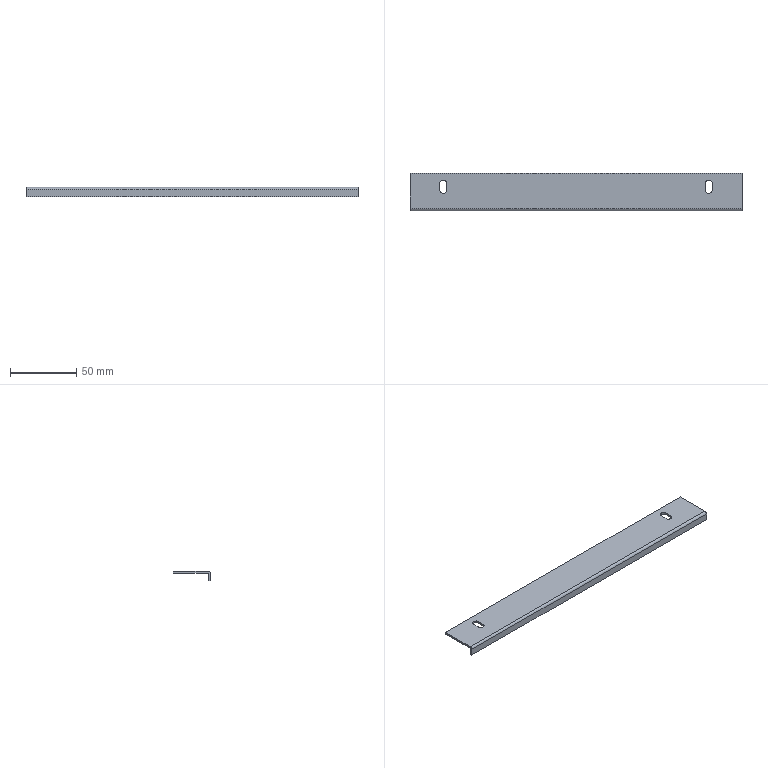Part | STEP file | FHD-021-014-02 acrylic press plate | 1 solid | 18 faces | box 250 x 28 x 7 mm | volume 12276 mm3 | plane 12 | cylinder 6 | commonest cylinder face diameters 5 x4 0.4 x1 3.4 x1
STEP:
#1=CARTESIAN_POINT('',(0.,0.,0.));
#2=DIRECTION('',(0.,0.,1.));
#3=DIRECTION('',(1.,0.,0.));
#4=AXIS2_PLACEMENT_3D('',#1,#2,#3);
#5=CARTESIAN_POINT('',(-125.,-12.3,-1.5));
#6=VERTEX_POINT('',#5);
#7=CARTESIAN_POINT('',(-125.,14.,-1.5));
#8=VERTEX_POINT('',#7);
#9=CARTESIAN_POINT('',(-125.,0.,-1.5));
#10=DIRECTION('',(0.,1.,0.));
#11=VECTOR('',#10,1.);
#12=LINE('',#9,#11);
#13=CARTESIAN_POINT('',(0.,0.,-1.5));
#14=DIRECTION('',(0.,0.,-1.));
#15=DIRECTION('',(-1.,0.,0.));
#16=AXIS2_PLACEMENT_3D('',#13,#14,#15);
#17=PLANE('',#16);
#18=CARTESIAN_POINT('',(125.,0.));
#19=DIRECTION('',(0.,1.));
#20=VECTOR('',#19,1.);
#21=LINE('',#18,#20);
#22=(GEOMETRIC_REPRESENTATION_CONTEXT(2)PARAMETRIC_REPRESENTATION_CONTEXT()REPRESENTATION_CONTEXT('',''));
#23=DEFINITIONAL_REPRESENTATION('',(#21),#22);
#24=PCURVE('',#17,#23);
#25=CARTESIAN_POINT('',(-125.,-14.,-1.5));
#26=DIRECTION('',(-1.,0.,0.));
#27=DIRECTION('',(0.,0.,1.));
#28=AXIS2_PLACEMENT_3D('',#25,#26,#27);
#29=PLANE('',#28);
#30=CARTESIAN_POINT('',(0.,14.));
#31=DIRECTION('',(0.,1.));
#32=VECTOR('',#31,1.);
#33=LINE('',#30,#32);
#34=(GEOMETRIC_REPRESENTATION_CONTEXT(2)PARAMETRIC_REPRESENTATION_CONTEXT()REPRESENTATION_CONTEXT('',''));
#35=DEFINITIONAL_REPRESENTATION('',(#33),#34);
#36=PCURVE('',#29,#35);
#37=SURFACE_CURVE('',#12,(#24,#36),.PCURVE_S1.);
#38=EDGE_CURVE('',#6,#8,#37,.T.);
#39=ORIENTED_EDGE('',*,*,#38,.T.);
#40=CARTESIAN_POINT('',(125.,14.,-1.5));
#41=VERTEX_POINT('',#40);
#42=CARTESIAN_POINT('',(0.,14.,-1.5));
#43=DIRECTION('',(1.,0.,0.));
#44=VECTOR('',#43,1.);
#45=LINE('',#42,#44);
#46=CARTESIAN_POINT('',(0.,14.));
#47=DIRECTION('',(-1.,0.));
#48=VECTOR('',#47,1.);
#49=LINE('',#46,#48);
#50=(GEOMETRIC_REPRESENTATION_CONTEXT(2)PARAMETRIC_REPRESENTATION_CONTEXT()REPRESENTATION_CONTEXT('',''));
#51=DEFINITIONAL_REPRESENTATION('',(#49),#50);
#52=PCURVE('',#17,#51);
#53=CARTESIAN_POINT('',(-125.,14.,-1.5));
#54=DIRECTION('',(0.,1.,0.));
#55=DIRECTION('',(0.,0.,1.));
#56=AXIS2_PLACEMENT_3D('',#53,#54,#55);
#57=PLANE('',#56);
#58=CARTESIAN_POINT('',(0.,125.));
#59=DIRECTION('',(0.,1.));
#60=VECTOR('',#59,1.);
#61=LINE('',#58,#60);
#62=(GEOMETRIC_REPRESENTATION_CONTEXT(2)PARAMETRIC_REPRESENTATION_CONTEXT()REPRESENTATION_CONTEXT('',''));
#63=DEFINITIONAL_REPRESENTATION('',(#61),#62);
#64=PCURVE('',#57,#63);
#65=SURFACE_CURVE('',#45,(#52,#64),.PCURVE_S1.);
#66=EDGE_CURVE('',#8,#41,#65,.T.);
#67=ORIENTED_EDGE('',*,*,#66,.T.);
#68=CARTESIAN_POINT('',(125.,-12.3,-1.5));
#69=VERTEX_POINT('',#68);
#70=CARTESIAN_POINT('',(125.,0.,-1.5));
#71=DIRECTION('',(0.,-1.,0.));
#72=VECTOR('',#71,1.);
#73=LINE('',#70,#72);
#74=CARTESIAN_POINT('',(-125.,0.));
#75=DIRECTION('',(0.,-1.));
#76=VECTOR('',#75,1.);
#77=LINE('',#74,#76);
#78=(GEOMETRIC_REPRESENTATION_CONTEXT(2)PARAMETRIC_REPRESENTATION_CONTEXT()REPRESENTATION_CONTEXT('',''));
#79=DEFINITIONAL_REPRESENTATION('',(#77),#78);
#80=PCURVE('',#17,#79);
#81=CARTESIAN_POINT('',(125.,-14.,-1.5));
#82=DIRECTION('',(1.,0.,0.));
#83=DIRECTION('',(0.,0.,-1.));
#84=AXIS2_PLACEMENT_3D('',#81,#82,#83);
#85=PLANE('',#84);
#86=CARTESIAN_POINT('',(0.,14.));
#87=DIRECTION('',(0.,-1.));
#88=VECTOR('',#87,1.);
#89=LINE('',#86,#88);
#90=(GEOMETRIC_REPRESENTATION_CONTEXT(2)PARAMETRIC_REPRESENTATION_CONTEXT()REPRESENTATION_CONTEXT('',''));
#91=DEFINITIONAL_REPRESENTATION('',(#89),#90);
#92=PCURVE('',#85,#91);
#93=SURFACE_CURVE('',#73,(#80,#92),.PCURVE_S1.);
#94=EDGE_CURVE('',#41,#69,#93,.T.);
#95=ORIENTED_EDGE('',*,*,#94,.T.);
#96=CARTESIAN_POINT('',(0.,-12.3,-1.5));
#97=DIRECTION('',(-1.,0.,0.));
#98=VECTOR('',#97,1.);
#99=LINE('',#96,#98);
#100=CARTESIAN_POINT('',(0.,-12.3));
#101=DIRECTION('',(1.,0.));
#102=VECTOR('',#101,1.);
#103=LINE('',#100,#102);
#104=(GEOMETRIC_REPRESENTATION_CONTEXT(2)PARAMETRIC_REPRESENTATION_CONTEXT()REPRESENTATION_CONTEXT('',''));
#105=DEFINITIONAL_REPRESENTATION('',(#103),#104);
#106=PCURVE('',#17,#105);
#107=CARTESIAN_POINT('',(-125.,-12.3,-1.7));
#108=DIRECTION('',(-1.,0.,0.));
#109=DIRECTION('',(0.,0.,1.));
#110=AXIS2_PLACEMENT_3D('',#107,#108,#109);
#111=CYLINDRICAL_SURFACE('',#110,0.2);
#112=CARTESIAN_POINT('',(6.283,-125.));
#113=DIRECTION('',(0.,1.));
#114=VECTOR('',#113,1.);
#115=LINE('',#112,#114);
#116=(GEOMETRIC_REPRESENTATION_CONTEXT(2)PARAMETRIC_REPRESENTATION_CONTEXT()REPRESENTATION_CONTEXT('',''));
#117=DEFINITIONAL_REPRESENTATION('',(#115),#116);
#118=PCURVE('',#111,#117);
#119=SURFACE_CURVE('',#99,(#106,#118),.PCURVE_S1.);
#120=EDGE_CURVE('',#69,#6,#119,.T.);
#121=ORIENTED_EDGE('',*,*,#120,.T.);
#122=EDGE_LOOP('',(#39,#67,#95,#121));
#123=FACE_BOUND('',#122,.T.);
#124=CARTESIAN_POINT('',(-102.5,1.5,-1.5));
#125=VERTEX_POINT('',#124);
#126=CARTESIAN_POINT('',(-97.5,1.5,-1.5));
#127=VERTEX_POINT('',#126);
#128=CARTESIAN_POINT('',(-100.,1.5,-1.5));
#129=DIRECTION('',(0.,0.,1.));
#130=DIRECTION('',(1.,0.,0.));
#131=AXIS2_PLACEMENT_3D('',#128,#129,#130);
#132=CIRCLE('',#131,2.5);
#133=CARTESIAN_POINT('',(97.5,1.5));
#134=CARTESIAN_POINT('',(97.5,5.83));
#135=CARTESIAN_POINT('',(101.25,3.665));
#136=CARTESIAN_POINT('',(105.,1.5));
#137=CARTESIAN_POINT('',(101.25,-0.6651));
#138=CARTESIAN_POINT('',(97.5,-2.83));
#139=CARTESIAN_POINT('',(97.5,1.5));
#140=(BOUNDED_CURVE()B_SPLINE_CURVE(2,(#133,#134,#135,#136,#137,#138,#139),.UNSPECIFIED.,.T.,.F.)B_SPLINE_CURVE_WITH_KNOTS((1,2,2,2,2,1),(-2.094,0.,2.094,4.189,6.283,8.378),.UNSPECIFIED.)CURVE()GEOMETRIC_REPRESENTATION_ITEM()RATIONAL_B_SPLINE_CURVE((1.,0.5,1.,0.5,1.,0.5,1.))REPRESENTATION_ITEM(''));
#141=(GEOMETRIC_REPRESENTATION_CONTEXT(2)PARAMETRIC_REPRESENTATION_CONTEXT()REPRESENTATION_CONTEXT('',''));
#142=DEFINITIONAL_REPRESENTATION('',(#140),#141);
#143=PCURVE('',#17,#142);
#144=CARTESIAN_POINT('',(-100.,1.5,-10.));
#145=DIRECTION('',(0.,0.,1.));
#146=DIRECTION('',(1.,0.,0.));
#147=AXIS2_PLACEMENT_3D('',#144,#145,#146);
#148=CYLINDRICAL_SURFACE('',#147,2.5);
#149=CARTESIAN_POINT('',(0.,8.5));
#150=DIRECTION('',(1.,0.));
#151=VECTOR('',#150,1.);
#152=LINE('',#149,#151);
#153=(GEOMETRIC_REPRESENTATION_CONTEXT(2)PARAMETRIC_REPRESENTATION_CONTEXT()REPRESENTATION_CONTEXT('',''));
#154=DEFINITIONAL_REPRESENTATION('',(#152),#153);
#155=PCURVE('',#148,#154);
#156=SURFACE_CURVE('',#132,(#143,#155),.PCURVE_S1.);
#157=EDGE_CURVE('',#125,#127,#156,.T.);
#158=ORIENTED_EDGE('',*,*,#157,.T.);
#159=CARTESIAN_POINT('',(-97.5,6.5,-1.5));
#160=VERTEX_POINT('',#159);
#161=CARTESIAN_POINT('',(-97.5,0.,-1.5));
#162=DIRECTION('',(0.,1.,0.));
#163=VECTOR('',#162,1.);
#164=LINE('',#161,#163);
#165=CARTESIAN_POINT('',(97.5,0.));
#166=DIRECTION('',(0.,1.));
#167=VECTOR('',#166,1.);
#168=LINE('',#165,#167);
#169=(GEOMETRIC_REPRESENTATION_CONTEXT(2)PARAMETRIC_REPRESENTATION_CONTEXT()REPRESENTATION_CONTEXT('',''));
#170=DEFINITIONAL_REPRESENTATION('',(#168),#169);
#171=PCURVE('',#17,#170);
#172=CARTESIAN_POINT('',(-97.5,6.5,-10.));
#173=DIRECTION('',(1.,0.,0.));
#174=DIRECTION('',(0.,0.,-1.));
#175=AXIS2_PLACEMENT_3D('',#172,#173,#174);
#176=PLANE('',#175);
#177=CARTESIAN_POINT('',(-8.5,-6.5));
#178=DIRECTION('',(0.,1.));
#179=VECTOR('',#178,1.);
#180=LINE('',#177,#179);
#181=(GEOMETRIC_REPRESENTATION_CONTEXT(2)PARAMETRIC_REPRESENTATION_CONTEXT()REPRESENTATION_CONTEXT('',''));
#182=DEFINITIONAL_REPRESENTATION('',(#180),#181);
#183=PCURVE('',#176,#182);
#184=SURFACE_CURVE('',#164,(#171,#183),.PCURVE_S1.);
#185=EDGE_CURVE('',#127,#160,#184,.T.);
#186=ORIENTED_EDGE('',*,*,#185,.T.);
#187=CARTESIAN_POINT('',(-102.5,6.5,-1.5));
#188=VERTEX_POINT('',#187);
#189=CARTESIAN_POINT('',(-100.,6.5,-1.5));
#190=DIRECTION('',(0.,0.,1.));
#191=DIRECTION('',(1.,0.,0.));
#192=AXIS2_PLACEMENT_3D('',#189,#190,#191);
#193=CIRCLE('',#192,2.5);
#194=CARTESIAN_POINT('',(97.5,6.5));
#195=CARTESIAN_POINT('',(97.5,10.83));
#196=CARTESIAN_POINT('',(101.25,8.665));
#197=CARTESIAN_POINT('',(105.,6.5));
#198=CARTESIAN_POINT('',(101.25,4.335));
#199=CARTESIAN_POINT('',(97.5,2.17));
#200=CARTESIAN_POINT('',(97.5,6.5));
#201=(BOUNDED_CURVE()B_SPLINE_CURVE(2,(#194,#195,#196,#197,#198,#199,#200),.UNSPECIFIED.,.T.,.F.)B_SPLINE_CURVE_WITH_KNOTS((1,2,2,2,2,1),(-2.094,0.,2.094,4.189,6.283,8.378),.UNSPECIFIED.)CURVE()GEOMETRIC_REPRESENTATION_ITEM()RATIONAL_B_SPLINE_CURVE((1.,0.5,1.,0.5,1.,0.5,1.))REPRESENTATION_ITEM(''));
#202=(GEOMETRIC_REPRESENTATION_CONTEXT(2)PARAMETRIC_REPRESENTATION_CONTEXT()REPRESENTATION_CONTEXT('',''));
#203=DEFINITIONAL_REPRESENTATION('',(#201),#202);
#204=PCURVE('',#17,#203);
#205=CARTESIAN_POINT('',(-100.,6.5,-10.));
#206=DIRECTION('',(0.,0.,1.));
#207=DIRECTION('',(1.,0.,0.));
#208=AXIS2_PLACEMENT_3D('',#205,#206,#207);
#209=CYLINDRICAL_SURFACE('',#208,2.5);
#210=CARTESIAN_POINT('',(0.,8.5));
#211=DIRECTION('',(1.,0.));
#212=VECTOR('',#211,1.);
#213=LINE('',#210,#212);
#214=(GEOMETRIC_REPRESENTATION_CONTEXT(2)PARAMETRIC_REPRESENTATION_CONTEXT()REPRESENTATION_CONTEXT('',''));
#215=DEFINITIONAL_REPRESENTATION('',(#213),#214);
#216=PCURVE('',#209,#215);
#217=SURFACE_CURVE('',#193,(#204,#216),.PCURVE_S1.);
#218=EDGE_CURVE('',#160,#188,#217,.T.);
#219=ORIENTED_EDGE('',*,*,#218,.T.);
#220=CARTESIAN_POINT('',(-102.5,0.,-1.5));
#221=DIRECTION('',(0.,-1.,0.));
#222=VECTOR('',#221,1.);
#223=LINE('',#220,#222);
#224=CARTESIAN_POINT('',(102.5,0.));
#225=DIRECTION('',(0.,-1.));
#226=VECTOR('',#225,1.);
#227=LINE('',#224,#226);
#228=(GEOMETRIC_REPRESENTATION_CONTEXT(2)PARAMETRIC_REPRESENTATION_CONTEXT()REPRESENTATION_CONTEXT('',''));
#229=DEFINITIONAL_REPRESENTATION('',(#227),#228);
#230=PCURVE('',#17,#229);
#231=CARTESIAN_POINT('',(-102.5,6.5,-10.));
#232=DIRECTION('',(-1.,0.,0.));
#233=DIRECTION('',(0.,0.,1.));
#234=AXIS2_PLACEMENT_3D('',#231,#232,#233);
#235=PLANE('',#234);
#236=CARTESIAN_POINT('',(8.5,-6.5));
#237=DIRECTION('',(0.,-1.));
#238=VECTOR('',#237,1.);
#239=LINE('',#236,#238);
#240=(GEOMETRIC_REPRESENTATION_CONTEXT(2)PARAMETRIC_REPRESENTATION_CONTEXT()REPRESENTATION_CONTEXT('',''));
#241=DEFINITIONAL_REPRESENTATION('',(#239),#240);
#242=PCURVE('',#235,#241);
#243=SURFACE_CURVE('',#223,(#230,#242),.PCURVE_S1.);
#244=EDGE_CURVE('',#188,#125,#243,.T.);
#245=ORIENTED_EDGE('',*,*,#244,.T.);
#246=EDGE_LOOP('',(#158,#186,#219,#245));
#247=FACE_BOUND('',#246,.T.);
#248=CARTESIAN_POINT('',(97.5,1.5,-1.5));
#249=VERTEX_POINT('',#248);
#250=CARTESIAN_POINT('',(102.5,1.5,-1.5));
#251=VERTEX_POINT('',#250);
#252=CARTESIAN_POINT('',(100.,1.5,-1.5));
#253=DIRECTION('',(0.,0.,1.));
#254=DIRECTION('',(1.,0.,0.));
#255=AXIS2_PLACEMENT_3D('',#252,#253,#254);
#256=CIRCLE('',#255,2.5);
#257=CARTESIAN_POINT('',(-102.5,1.5));
#258=CARTESIAN_POINT('',(-102.5,5.83));
#259=CARTESIAN_POINT('',(-98.75,3.665));
#260=CARTESIAN_POINT('',(-95.,1.5));
#261=CARTESIAN_POINT('',(-98.75,-0.6651));
#262=CARTESIAN_POINT('',(-102.5,-2.83));
#263=CARTESIAN_POINT('',(-102.5,1.5));
#264=(BOUNDED_CURVE()B_SPLINE_CURVE(2,(#257,#258,#259,#260,#261,#262,#263),.UNSPECIFIED.,.T.,.F.)B_SPLINE_CURVE_WITH_KNOTS((1,2,2,2,2,1),(-2.094,0.,2.094,4.189,6.283,8.378),.UNSPECIFIED.)CURVE()GEOMETRIC_REPRESENTATION_ITEM()RATIONAL_B_SPLINE_CURVE((1.,0.5,1.,0.5,1.,0.5,1.))REPRESENTATION_ITEM(''));
#265=(GEOMETRIC_REPRESENTATION_CONTEXT(2)PARAMETRIC_REPRESENTATION_CONTEXT()REPRESENTATION_CONTEXT('',''));
#266=DEFINITIONAL_REPRESENTATION('',(#264),#265);
#267=PCURVE('',#17,#266);
#268=CARTESIAN_POINT('',(100.,1.5,-10.));
#269=DIRECTION('',(0.,0.,1.));
#270=DIRECTION('',(1.,0.,0.));
#271=AXIS2_PLACEMENT_3D('',#268,#269,#270);
#272=CYLINDRICAL_SURFACE('',#271,2.5);
#273=CARTESIAN_POINT('',(0.,8.5));
#274=DIRECTION('',(1.,0.));
#275=VECTOR('',#274,1.);
#276=LINE('',#273,#275);
#277=(GEOMETRIC_REPRESENTATION_CONTEXT(2)PARAMETRIC_REPRESENTATION_CONTEXT()REPRESENTATION_CONTEXT('',''));
#278=DEFINITIONAL_REPRESENTATION('',(#276),#277);
#279=PCURVE('',#272,#278);
#280=SURFACE_CURVE('',#256,(#267,#279),.PCURVE_S1.);
#281=EDGE_CURVE('',#249,#251,#280,.T.);
#282=ORIENTED_EDGE('',*,*,#281,.T.);
#283=CARTESIAN_POINT('',(102.5,6.5,-1.5));
#284=VERTEX_POINT('',#283);
#285=CARTESIAN_POINT('',(102.5,0.,-1.5));
#286=DIRECTION('',(0.,1.,0.));
#287=VECTOR('',#286,1.);
#288=LINE('',#285,#287);
#289=CARTESIAN_POINT('',(-102.5,0.));
#290=DIRECTION('',(0.,1.));
#291=VECTOR('',#290,1.);
#292=LINE('',#289,#291);
#293=(GEOMETRIC_REPRESENTATION_CONTEXT(2)PARAMETRIC_REPRESENTATION_CONTEXT()REPRESENTATION_CONTEXT('',''));
#294=DEFINITIONAL_REPRESENTATION('',(#292),#293);
#295=PCURVE('',#17,#294);
#296=CARTESIAN_POINT('',(102.5,6.5,-10.));
#297=DIRECTION('',(1.,0.,0.));
#298=DIRECTION('',(0.,0.,-1.));
#299=AXIS2_PLACEMENT_3D('',#296,#297,#298);
#300=PLANE('',#299);
#301=CARTESIAN_POINT('',(-8.5,-6.5));
#302=DIRECTION('',(0.,1.));
#303=VECTOR('',#302,1.);
#304=LINE('',#301,#303);
#305=(GEOMETRIC_REPRESENTATION_CONTEXT(2)PARAMETRIC_REPRESENTATION_CONTEXT()REPRESENTATION_CONTEXT('',''));
#306=DEFINITIONAL_REPRESENTATION('',(#304),#305);
#307=PCURVE('',#300,#306);
#308=SURFACE_CURVE('',#288,(#295,#307),.PCURVE_S1.);
#309=EDGE_CURVE('',#251,#284,#308,.T.);
#310=ORIENTED_EDGE('',*,*,#309,.T.);
#311=CARTESIAN_POINT('',(97.5,6.5,-1.5));
#312=VERTEX_POINT('',#311);
#313=CARTESIAN_POINT('',(100.,6.5,-1.5));
#314=DIRECTION('',(0.,0.,1.));
#315=DIRECTION('',(1.,0.,0.));
#316=AXIS2_PLACEMENT_3D('',#313,#314,#315);
#317=CIRCLE('',#316,2.5);
#318=CARTESIAN_POINT('',(-102.5,6.5));
#319=CARTESIAN_POINT('',(-102.5,10.83));
#320=CARTESIAN_POINT('',(-98.75,8.665));
#321=CARTESIAN_POINT('',(-95.,6.5));
#322=CARTESIAN_POINT('',(-98.75,4.335));
#323=CARTESIAN_POINT('',(-102.5,2.17));
#324=CARTESIAN_POINT('',(-102.5,6.5));
#325=(BOUNDED_CURVE()B_SPLINE_CURVE(2,(#318,#319,#320,#321,#322,#323,#324),.UNSPECIFIED.,.T.,.F.)B_SPLINE_CURVE_WITH_KNOTS((1,2,2,2,2,1),(-2.094,0.,2.094,4.189,6.283,8.378),.UNSPECIFIED.)CURVE()GEOMETRIC_REPRESENTATION_ITEM()RATIONAL_B_SPLINE_CURVE((1.,0.5,1.,0.5,1.,0.5,1.))REPRESENTATION_ITEM(''));
#326=(GEOMETRIC_REPRESENTATION_CONTEXT(2)PARAMETRIC_REPRESENTATION_CONTEXT()REPRESENTATION_CONTEXT('',''));
#327=DEFINITIONAL_REPRESENTATION('',(#325),#326);
#328=PCURVE('',#17,#327);
#329=CARTESIAN_POINT('',(100.,6.5,-10.));
#330=DIRECTION('',(0.,0.,1.));
#331=DIRECTION('',(1.,0.,0.));
#332=AXIS2_PLACEMENT_3D('',#329,#330,#331);
#333=CYLINDRICAL_SURFACE('',#332,2.5);
#334=CARTESIAN_POINT('',(0.,8.5));
#335=DIRECTION('',(1.,0.));
#336=VECTOR('',#335,1.);
#337=LINE('',#334,#336);
#338=(GEOMETRIC_REPRESENTATION_CONTEXT(2)PARAMETRIC_REPRESENTATION_CONTEXT()REPRESENTATION_CONTEXT('',''));
#339=DEFINITIONAL_REPRESENTATION('',(#337),#338);
#340=PCURVE('',#333,#339);
#341=SURFACE_CURVE('',#317,(#328,#340),.PCURVE_S1.);
#342=EDGE_CURVE('',#284,#312,#341,.T.);
#343=ORIENTED_EDGE('',*,*,#342,.T.);
#344=CARTESIAN_POINT('',(97.5,0.,-1.5));
#345=DIRECTION('',(0.,-1.,0.));
#346=VECTOR('',#345,1.);
#347=LINE('',#344,#346);
#348=CARTESIAN_POINT('',(-97.5,0.));
#349=DIRECTION('',(0.,-1.));
#350=VECTOR('',#349,1.);
#351=LINE('',#348,#350);
#352=(GEOMETRIC_REPRESENTATION_CONTEXT(2)PARAMETRIC_REPRESENTATION_CONTEXT()REPRESENTATION_CONTEXT('',''));
#353=DEFINITIONAL_REPRESENTATION('',(#351),#352);
#354=PCURVE('',#17,#353);
#355=CARTESIAN_POINT('',(97.5,6.5,-10.));
#356=DIRECTION('',(-1.,0.,0.));
#357=DIRECTION('',(0.,0.,1.));
#358=AXIS2_PLACEMENT_3D('',#355,#356,#357);
#359=PLANE('',#358);
#360=CARTESIAN_POINT('',(8.5,-6.5));
#361=DIRECTION('',(0.,-1.));
#362=VECTOR('',#361,1.);
#363=LINE('',#360,#362);
#364=(GEOMETRIC_REPRESENTATION_CONTEXT(2)PARAMETRIC_REPRESENTATION_CONTEXT()REPRESENTATION_CONTEXT('',''));
#365=DEFINITIONAL_REPRESENTATION('',(#363),#364);
#366=PCURVE('',#359,#365);
#367=SURFACE_CURVE('',#347,(#354,#366),.PCURVE_S1.);
#368=EDGE_CURVE('',#312,#249,#367,.T.);
#369=ORIENTED_EDGE('',*,*,#368,.T.);
#370=EDGE_LOOP('',(#282,#310,#343,#369));
#371=FACE_BOUND('',#370,.T.);
#372=ADVANCED_FACE('',(#123,#247,#371),#17,.T.);
#373=ORIENTED_EDGE('',*,*,#66,.F.);
#374=CARTESIAN_POINT('',(-125.,14.,0.));
#375=VERTEX_POINT('',#374);
#376=CARTESIAN_POINT('',(-125.,14.,-1.5));
#377=DIRECTION('',(0.,0.,1.));
#378=VECTOR('',#377,1.);
#379=LINE('',#376,#378);
#380=CARTESIAN_POINT('',(0.,0.));
#381=DIRECTION('',(1.,0.));
#382=VECTOR('',#381,1.);
#383=LINE('',#380,#382);
#384=(GEOMETRIC_REPRESENTATION_CONTEXT(2)PARAMETRIC_REPRESENTATION_CONTEXT()REPRESENTATION_CONTEXT('',''));
#385=DEFINITIONAL_REPRESENTATION('',(#383),#384);
#386=PCURVE('',#57,#385);
#387=CARTESIAN_POINT('',(0.,28.));
#388=DIRECTION('',(1.,0.));
#389=VECTOR('',#388,1.);
#390=LINE('',#387,#389);
#391=(GEOMETRIC_REPRESENTATION_CONTEXT(2)PARAMETRIC_REPRESENTATION_CONTEXT()REPRESENTATION_CONTEXT('',''));
#392=DEFINITIONAL_REPRESENTATION('',(#390),#391);
#393=PCURVE('',#29,#392);
#394=SURFACE_CURVE('',#379,(#386,#393),.PCURVE_S1.);
#395=EDGE_CURVE('',#8,#375,#394,.T.);
#396=ORIENTED_EDGE('',*,*,#395,.T.);
#397=CARTESIAN_POINT('',(125.,14.,0.));
#398=VERTEX_POINT('',#397);
#399=CARTESIAN_POINT('',(-125.,14.,0.));
#400=DIRECTION('',(1.,0.,0.));
#401=VECTOR('',#400,1.);
#402=LINE('',#399,#401);
#403=CARTESIAN_POINT('',(1.5,0.));
#404=DIRECTION('',(0.,1.));
#405=VECTOR('',#404,1.);
#406=LINE('',#403,#405);
#407=(GEOMETRIC_REPRESENTATION_CONTEXT(2)PARAMETRIC_REPRESENTATION_CONTEXT()REPRESENTATION_CONTEXT('',''));
#408=DEFINITIONAL_REPRESENTATION('',(#406),#407);
#409=PCURVE('',#57,#408);
#410=CARTESIAN_POINT('',(0.,0.,0.));
#411=DIRECTION('',(0.,0.,-1.));
#412=DIRECTION('',(-1.,0.,0.));
#413=AXIS2_PLACEMENT_3D('',#410,#411,#412);
#414=PLANE('',#413);
#415=CARTESIAN_POINT('',(125.,14.));
#416=DIRECTION('',(-1.,0.));
#417=VECTOR('',#416,1.);
#418=LINE('',#415,#417);
#419=(GEOMETRIC_REPRESENTATION_CONTEXT(2)PARAMETRIC_REPRESENTATION_CONTEXT()REPRESENTATION_CONTEXT('',''));
#420=DEFINITIONAL_REPRESENTATION('',(#418),#419);
#421=PCURVE('',#414,#420);
#422=SURFACE_CURVE('',#402,(#409,#421),.PCURVE_S1.);
#423=EDGE_CURVE('',#375,#398,#422,.T.);
#424=ORIENTED_EDGE('',*,*,#423,.T.);
#425=CARTESIAN_POINT('',(125.,14.,-1.5));
#426=DIRECTION('',(0.,0.,-1.));
#427=VECTOR('',#426,1.);
#428=LINE('',#425,#427);
#429=CARTESIAN_POINT('',(0.,250.));
#430=DIRECTION('',(-1.,0.));
#431=VECTOR('',#430,1.);
#432=LINE('',#429,#431);
#433=(GEOMETRIC_REPRESENTATION_CONTEXT(2)PARAMETRIC_REPRESENTATION_CONTEXT()REPRESENTATION_CONTEXT('',''));
#434=DEFINITIONAL_REPRESENTATION('',(#432),#433);
#435=PCURVE('',#57,#434);
#436=CARTESIAN_POINT('',(0.,28.));
#437=DIRECTION('',(1.,0.));
#438=VECTOR('',#437,1.);
#439=LINE('',#436,#438);
#440=(GEOMETRIC_REPRESENTATION_CONTEXT(2)PARAMETRIC_REPRESENTATION_CONTEXT()REPRESENTATION_CONTEXT('',''));
#441=DEFINITIONAL_REPRESENTATION('',(#439),#440);
#442=PCURVE('',#85,#441);
#443=SURFACE_CURVE('',#428,(#435,#442),.PCURVE_S1.);
#444=EDGE_CURVE('',#398,#41,#443,.T.);
#445=ORIENTED_EDGE('',*,*,#444,.T.);
#446=EDGE_LOOP('',(#373,#396,#424,#445));
#447=FACE_BOUND('',#446,.T.);
#448=ADVANCED_FACE('',(#447),#57,.T.);
#449=CARTESIAN_POINT('',(-125.,-12.3,0.));
#450=VERTEX_POINT('',#449);
#451=CARTESIAN_POINT('',(-125.,-14.,0.));
#452=DIRECTION('',(0.,1.,0.));
#453=VECTOR('',#452,1.);
#454=LINE('',#451,#453);
#455=CARTESIAN_POINT('',(1.5,0.));
#456=DIRECTION('',(0.,1.));
#457=VECTOR('',#456,1.);
#458=LINE('',#455,#457);
#459=(GEOMETRIC_REPRESENTATION_CONTEXT(2)PARAMETRIC_REPRESENTATION_CONTEXT()REPRESENTATION_CONTEXT('',''));
#460=DEFINITIONAL_REPRESENTATION('',(#458),#459);
#461=PCURVE('',#29,#460);
#462=CARTESIAN_POINT('',(125.,-14.));
#463=DIRECTION('',(0.,1.));
#464=VECTOR('',#463,1.);
#465=LINE('',#462,#464);
#466=(GEOMETRIC_REPRESENTATION_CONTEXT(2)PARAMETRIC_REPRESENTATION_CONTEXT()REPRESENTATION_CONTEXT('',''));
#467=DEFINITIONAL_REPRESENTATION('',(#465),#466);
#468=PCURVE('',#414,#467);
#469=SURFACE_CURVE('',#454,(#461,#468),.PCURVE_S1.);
#470=EDGE_CURVE('',#450,#375,#469,.T.);
#471=ORIENTED_EDGE('',*,*,#470,.T.);
#472=ORIENTED_EDGE('',*,*,#395,.F.);
#473=ORIENTED_EDGE('',*,*,#38,.F.);
#474=CARTESIAN_POINT('',(-125.,-12.5,-1.7));
#475=VERTEX_POINT('',#474);
#476=CARTESIAN_POINT('',(-125.,-12.3,-1.7));
#477=DIRECTION('',(-1.,0.,0.));
#478=DIRECTION('',(0.,0.,1.));
#479=AXIS2_PLACEMENT_3D('',#476,#477,#478);
#480=CIRCLE('',#479,0.2);
#481=CARTESIAN_POINT('',(-0.2,1.7));
#482=DIRECTION('',(1.,0.));
#483=AXIS2_PLACEMENT_2D('',#481,#482);
#484=CIRCLE('',#483,0.2);
#485=(GEOMETRIC_REPRESENTATION_CONTEXT(2)PARAMETRIC_REPRESENTATION_CONTEXT()REPRESENTATION_CONTEXT('',''));
#486=DEFINITIONAL_REPRESENTATION('',(#484),#485);
#487=PCURVE('',#29,#486);
#488=CARTESIAN_POINT('',(0.,0.));
#489=DIRECTION('',(1.,0.));
#490=VECTOR('',#489,1.);
#491=LINE('',#488,#490);
#492=(GEOMETRIC_REPRESENTATION_CONTEXT(2)PARAMETRIC_REPRESENTATION_CONTEXT()REPRESENTATION_CONTEXT('',''));
#493=DEFINITIONAL_REPRESENTATION('',(#491),#492);
#494=PCURVE('',#111,#493);
#495=SURFACE_CURVE('',#480,(#487,#494),.PCURVE_S1.);
#496=EDGE_CURVE('',#475,#6,#495,.T.);
#497=ORIENTED_EDGE('',*,*,#496,.F.);
#498=CARTESIAN_POINT('',(-125.,-12.5,-7.));
#499=VERTEX_POINT('',#498);
#500=CARTESIAN_POINT('',(-125.,-12.5,0.));
#501=DIRECTION('',(0.,0.,1.));
#502=VECTOR('',#501,1.);
#503=LINE('',#500,#502);
#504=CARTESIAN_POINT('',(1.5,1.5));
#505=DIRECTION('',(1.,0.));
#506=VECTOR('',#505,1.);
#507=LINE('',#504,#506);
#508=(GEOMETRIC_REPRESENTATION_CONTEXT(2)PARAMETRIC_REPRESENTATION_CONTEXT()REPRESENTATION_CONTEXT('',''));
#509=DEFINITIONAL_REPRESENTATION('',(#507),#508);
#510=PCURVE('',#29,#509);
#511=CARTESIAN_POINT('',(0.,-12.5,0.));
#512=DIRECTION('',(0.,1.,0.));
#513=DIRECTION('',(0.,0.,1.));
#514=AXIS2_PLACEMENT_3D('',#511,#512,#513);
#515=PLANE('',#514);
#516=CARTESIAN_POINT('',(0.,-125.));
#517=DIRECTION('',(1.,0.));
#518=VECTOR('',#517,1.);
#519=LINE('',#516,#518);
#520=(GEOMETRIC_REPRESENTATION_CONTEXT(2)PARAMETRIC_REPRESENTATION_CONTEXT()REPRESENTATION_CONTEXT('',''));
#521=DEFINITIONAL_REPRESENTATION('',(#519),#520);
#522=PCURVE('',#515,#521);
#523=SURFACE_CURVE('',#503,(#510,#522),.PCURVE_S1.);
#524=EDGE_CURVE('',#499,#475,#523,.T.);
#525=ORIENTED_EDGE('',*,*,#524,.F.);
#526=CARTESIAN_POINT('',(-125.,-14.,-7.));
#527=VERTEX_POINT('',#526);
#528=CARTESIAN_POINT('',(-125.,-14.,-7.));
#529=DIRECTION('',(0.,-1.,0.));
#530=VECTOR('',#529,1.);
#531=LINE('',#528,#530);
#532=CARTESIAN_POINT('',(-5.5,0.));
#533=DIRECTION('',(0.,-1.));
#534=VECTOR('',#533,1.);
#535=LINE('',#532,#534);
#536=(GEOMETRIC_REPRESENTATION_CONTEXT(2)PARAMETRIC_REPRESENTATION_CONTEXT()REPRESENTATION_CONTEXT('',''));
#537=DEFINITIONAL_REPRESENTATION('',(#535),#536);
#538=PCURVE('',#29,#537);
#539=CARTESIAN_POINT('',(125.,-14.,-7.));
#540=DIRECTION('',(0.,0.,1.));
#541=DIRECTION('',(0.,-1.,0.));
#542=AXIS2_PLACEMENT_3D('',#539,#540,#541);
#543=PLANE('',#542);
#544=CARTESIAN_POINT('',(0.,-250.));
#545=DIRECTION('',(1.,0.));
#546=VECTOR('',#545,1.);
#547=LINE('',#544,#546);
#548=(GEOMETRIC_REPRESENTATION_CONTEXT(2)PARAMETRIC_REPRESENTATION_CONTEXT()REPRESENTATION_CONTEXT('',''));
#549=DEFINITIONAL_REPRESENTATION('',(#547),#548);
#550=PCURVE('',#543,#549);
#551=SURFACE_CURVE('',#531,(#538,#550),.PCURVE_S1.);
#552=EDGE_CURVE('',#499,#527,#551,.T.);
#553=ORIENTED_EDGE('',*,*,#552,.T.);
#554=CARTESIAN_POINT('',(-125.,-14.,-1.7));
#555=VERTEX_POINT('',#554);
#556=CARTESIAN_POINT('',(-125.,-14.,-7.));
#557=DIRECTION('',(0.,0.,-1.));
#558=VECTOR('',#557,1.);
#559=LINE('',#556,#558);
#560=CARTESIAN_POINT('',(-5.5,0.));
#561=DIRECTION('',(-1.,0.));
#562=VECTOR('',#561,1.);
#563=LINE('',#560,#562);
#564=(GEOMETRIC_REPRESENTATION_CONTEXT(2)PARAMETRIC_REPRESENTATION_CONTEXT()REPRESENTATION_CONTEXT('',''));
#565=DEFINITIONAL_REPRESENTATION('',(#563),#564);
#566=PCURVE('',#29,#565);
#567=CARTESIAN_POINT('',(0.,-14.,0.));
#568=DIRECTION('',(0.,1.,0.));
#569=DIRECTION('',(0.,0.,1.));
#570=AXIS2_PLACEMENT_3D('',#567,#568,#569);
#571=PLANE('',#570);
#572=CARTESIAN_POINT('',(-7.,-125.));
#573=DIRECTION('',(-1.,0.));
#574=VECTOR('',#573,1.);
#575=LINE('',#572,#574);
#576=(GEOMETRIC_REPRESENTATION_CONTEXT(2)PARAMETRIC_REPRESENTATION_CONTEXT()REPRESENTATION_CONTEXT('',''));
#577=DEFINITIONAL_REPRESENTATION('',(#575),#576);
#578=PCURVE('',#571,#577);
#579=SURFACE_CURVE('',#559,(#566,#578),.PCURVE_S1.);
#580=EDGE_CURVE('',#555,#527,#579,.T.);
#581=ORIENTED_EDGE('',*,*,#580,.F.);
#582=CARTESIAN_POINT('',(-125.,-12.3,-1.7));
#583=DIRECTION('',(1.,0.,0.));
#584=DIRECTION('',(0.,0.,1.));
#585=AXIS2_PLACEMENT_3D('',#582,#583,#584);
#586=CIRCLE('',#585,1.7);
#587=CARTESIAN_POINT('',(1.5,1.7));
#588=CARTESIAN_POINT('',(1.5,-1.244));
#589=CARTESIAN_POINT('',(-1.05,0.2278));
#590=CARTESIAN_POINT('',(-3.6,1.7));
#591=CARTESIAN_POINT('',(-1.05,3.172));
#592=CARTESIAN_POINT('',(1.5,4.644));
#593=CARTESIAN_POINT('',(1.5,1.7));
#594=(BOUNDED_CURVE()B_SPLINE_CURVE(2,(#587,#588,#589,#590,#591,#592,#593),.UNSPECIFIED.,.T.,.F.)B_SPLINE_CURVE_WITH_KNOTS((1,2,2,2,2,1),(-2.094,0.,2.094,4.189,6.283,8.378),.UNSPECIFIED.)CURVE()GEOMETRIC_REPRESENTATION_ITEM()RATIONAL_B_SPLINE_CURVE((1.,0.5,1.,0.5,1.,0.5,1.))REPRESENTATION_ITEM(''));
#595=(GEOMETRIC_REPRESENTATION_CONTEXT(2)PARAMETRIC_REPRESENTATION_CONTEXT()REPRESENTATION_CONTEXT('',''));
#596=DEFINITIONAL_REPRESENTATION('',(#594),#595);
#597=PCURVE('',#29,#596);
#598=CARTESIAN_POINT('',(-125.,-12.3,-1.7));
#599=DIRECTION('',(-1.,0.,0.));
#600=DIRECTION('',(0.,0.,1.));
#601=AXIS2_PLACEMENT_3D('',#598,#599,#600);
#602=CYLINDRICAL_SURFACE('',#601,1.7);
#603=CARTESIAN_POINT('',(6.283,0.));
#604=DIRECTION('',(-1.,0.));
#605=VECTOR('',#604,1.);
#606=LINE('',#603,#605);
#607=(GEOMETRIC_REPRESENTATION_CONTEXT(2)PARAMETRIC_REPRESENTATION_CONTEXT()REPRESENTATION_CONTEXT('',''));
#608=DEFINITIONAL_REPRESENTATION('',(#606),#607);
#609=PCURVE('',#602,#608);
#610=SURFACE_CURVE('',#586,(#597,#609),.PCURVE_S1.);
#611=EDGE_CURVE('',#450,#555,#610,.T.);
#612=ORIENTED_EDGE('',*,*,#611,.F.);
#613=EDGE_LOOP('',(#471,#472,#473,#497,#525,#553,#581,#612));
#614=FACE_BOUND('',#613,.T.);
#615=ADVANCED_FACE('',(#614),#29,.T.);
#616=ORIENTED_EDGE('',*,*,#120,.T.);
#617=ORIENTED_EDGE('',*,*,#496,.F.);
#618=CARTESIAN_POINT('',(125.,-12.5,-1.7));
#619=VERTEX_POINT('',#618);
#620=CARTESIAN_POINT('',(-125.,-12.5,-1.7));
#621=DIRECTION('',(1.,0.,0.));
#622=VECTOR('',#621,1.);
#623=LINE('',#620,#622);
#624=CARTESIAN_POINT('',(4.712,0.));
#625=DIRECTION('',(0.,-1.));
#626=VECTOR('',#625,1.);
#627=LINE('',#624,#626);
#628=(GEOMETRIC_REPRESENTATION_CONTEXT(2)PARAMETRIC_REPRESENTATION_CONTEXT()REPRESENTATION_CONTEXT('',''));
#629=DEFINITIONAL_REPRESENTATION('',(#627),#628);
#630=PCURVE('',#111,#629);
#631=CARTESIAN_POINT('',(-1.7,-125.));
#632=DIRECTION('',(0.,1.));
#633=VECTOR('',#632,1.);
#634=LINE('',#631,#633);
#635=(GEOMETRIC_REPRESENTATION_CONTEXT(2)PARAMETRIC_REPRESENTATION_CONTEXT()REPRESENTATION_CONTEXT('',''));
#636=DEFINITIONAL_REPRESENTATION('',(#634),#635);
#637=PCURVE('',#515,#636);
#638=SURFACE_CURVE('',#623,(#630,#637),.PCURVE_S1.);
#639=EDGE_CURVE('',#475,#619,#638,.T.);
#640=ORIENTED_EDGE('',*,*,#639,.T.);
#641=CARTESIAN_POINT('',(125.,-12.3,-1.7));
#642=DIRECTION('',(-1.,0.,0.));
#643=DIRECTION('',(0.,0.,1.));
#644=AXIS2_PLACEMENT_3D('',#641,#642,#643);
#645=CIRCLE('',#644,0.2);
#646=CARTESIAN_POINT('',(0.,-250.));
#647=DIRECTION('',(1.,0.));
#648=VECTOR('',#647,1.);
#649=LINE('',#646,#648);
#650=(GEOMETRIC_REPRESENTATION_CONTEXT(2)PARAMETRIC_REPRESENTATION_CONTEXT()REPRESENTATION_CONTEXT('',''));
#651=DEFINITIONAL_REPRESENTATION('',(#649),#650);
#652=PCURVE('',#111,#651);
#653=CARTESIAN_POINT('',(0.,1.7));
#654=CARTESIAN_POINT('',(0.,2.046));
#655=CARTESIAN_POINT('',(0.3,1.873));
#656=CARTESIAN_POINT('',(0.6,1.7));
#657=CARTESIAN_POINT('',(0.3,1.527));
#658=CARTESIAN_POINT('',(0.,1.354));
#659=CARTESIAN_POINT('',(0.,1.7));
#660=(BOUNDED_CURVE()B_SPLINE_CURVE(2,(#653,#654,#655,#656,#657,#658,#659),.UNSPECIFIED.,.T.,.F.)B_SPLINE_CURVE_WITH_KNOTS((1,2,2,2,2,1),(-2.094,0.,2.094,4.189,6.283,8.378),.UNSPECIFIED.)CURVE()GEOMETRIC_REPRESENTATION_ITEM()RATIONAL_B_SPLINE_CURVE((1.,0.5,1.,0.5,1.,0.5,1.))REPRESENTATION_ITEM(''));
#661=(GEOMETRIC_REPRESENTATION_CONTEXT(2)PARAMETRIC_REPRESENTATION_CONTEXT()REPRESENTATION_CONTEXT('',''));
#662=DEFINITIONAL_REPRESENTATION('',(#660),#661);
#663=PCURVE('',#85,#662);
#664=SURFACE_CURVE('',#645,(#652,#663),.PCURVE_S1.);
#665=EDGE_CURVE('',#619,#69,#664,.T.);
#666=ORIENTED_EDGE('',*,*,#665,.T.);
#667=EDGE_LOOP('',(#616,#617,#640,#666));
#668=FACE_BOUND('',#667,.F.);
#669=ADVANCED_FACE('',(#668),#111,.F.);
#670=ORIENTED_EDGE('',*,*,#444,.F.);
#671=CARTESIAN_POINT('',(125.,-12.3,0.));
#672=VERTEX_POINT('',#671);
#673=CARTESIAN_POINT('',(125.,-14.,0.));
#674=DIRECTION('',(0.,-1.,0.));
#675=VECTOR('',#674,1.);
#676=LINE('',#673,#675);
#677=CARTESIAN_POINT('',(-1.5,0.));
#678=DIRECTION('',(0.,-1.));
#679=VECTOR('',#678,1.);
#680=LINE('',#677,#679);
#681=(GEOMETRIC_REPRESENTATION_CONTEXT(2)PARAMETRIC_REPRESENTATION_CONTEXT()REPRESENTATION_CONTEXT('',''));
#682=DEFINITIONAL_REPRESENTATION('',(#680),#681);
#683=PCURVE('',#85,#682);
#684=CARTESIAN_POINT('',(-125.,-14.));
#685=DIRECTION('',(0.,-1.));
#686=VECTOR('',#685,1.);
#687=LINE('',#684,#686);
#688=(GEOMETRIC_REPRESENTATION_CONTEXT(2)PARAMETRIC_REPRESENTATION_CONTEXT()REPRESENTATION_CONTEXT('',''));
#689=DEFINITIONAL_REPRESENTATION('',(#687),#688);
#690=PCURVE('',#414,#689);
#691=SURFACE_CURVE('',#676,(#683,#690),.PCURVE_S1.);
#692=EDGE_CURVE('',#398,#672,#691,.T.);
#693=ORIENTED_EDGE('',*,*,#692,.T.);
#694=CARTESIAN_POINT('',(125.,-14.,-1.7));
#695=VERTEX_POINT('',#694);
#696=CARTESIAN_POINT('',(125.,-12.3,-1.7));
#697=DIRECTION('',(-1.,0.,0.));
#698=DIRECTION('',(0.,0.,1.));
#699=AXIS2_PLACEMENT_3D('',#696,#697,#698);
#700=CIRCLE('',#699,1.7);
#701=CARTESIAN_POINT('',(-1.5,1.7));
#702=CARTESIAN_POINT('',(-1.5,4.644));
#703=CARTESIAN_POINT('',(1.05,3.172));
#704=CARTESIAN_POINT('',(3.6,1.7));
#705=CARTESIAN_POINT('',(1.05,0.2278));
#706=CARTESIAN_POINT('',(-1.5,-1.244));
#707=CARTESIAN_POINT('',(-1.5,1.7));
#708=(BOUNDED_CURVE()B_SPLINE_CURVE(2,(#701,#702,#703,#704,#705,#706,#707),.UNSPECIFIED.,.T.,.F.)B_SPLINE_CURVE_WITH_KNOTS((1,2,2,2,2,1),(-2.094,0.,2.094,4.189,6.283,8.378),.UNSPECIFIED.)CURVE()GEOMETRIC_REPRESENTATION_ITEM()RATIONAL_B_SPLINE_CURVE((1.,0.5,1.,0.5,1.,0.5,1.))REPRESENTATION_ITEM(''));
#709=(GEOMETRIC_REPRESENTATION_CONTEXT(2)PARAMETRIC_REPRESENTATION_CONTEXT()REPRESENTATION_CONTEXT('',''));
#710=DEFINITIONAL_REPRESENTATION('',(#708),#709);
#711=PCURVE('',#85,#710);
#712=CARTESIAN_POINT('',(0.,-250.));
#713=DIRECTION('',(1.,0.));
#714=VECTOR('',#713,1.);
#715=LINE('',#712,#714);
#716=(GEOMETRIC_REPRESENTATION_CONTEXT(2)PARAMETRIC_REPRESENTATION_CONTEXT()REPRESENTATION_CONTEXT('',''));
#717=DEFINITIONAL_REPRESENTATION('',(#715),#716);
#718=PCURVE('',#602,#717);
#719=SURFACE_CURVE('',#700,(#711,#718),.PCURVE_S1.);
#720=EDGE_CURVE('',#695,#672,#719,.T.);
#721=ORIENTED_EDGE('',*,*,#720,.F.);
#722=CARTESIAN_POINT('',(125.,-14.,-7.));
#723=VERTEX_POINT('',#722);
#724=CARTESIAN_POINT('',(125.,-14.,-1.5));
#725=DIRECTION('',(0.,0.,1.));
#726=VECTOR('',#725,1.);
#727=LINE('',#724,#726);
#728=CARTESIAN_POINT('',(0.,0.));
#729=DIRECTION('',(-1.,0.));
#730=VECTOR('',#729,1.);
#731=LINE('',#728,#730);
#732=(GEOMETRIC_REPRESENTATION_CONTEXT(2)PARAMETRIC_REPRESENTATION_CONTEXT()REPRESENTATION_CONTEXT('',''));
#733=DEFINITIONAL_REPRESENTATION('',(#731),#732);
#734=PCURVE('',#85,#733);
#735=CARTESIAN_POINT('',(-1.5,125.));
#736=DIRECTION('',(1.,0.));
#737=VECTOR('',#736,1.);
#738=LINE('',#735,#737);
#739=(GEOMETRIC_REPRESENTATION_CONTEXT(2)PARAMETRIC_REPRESENTATION_CONTEXT()REPRESENTATION_CONTEXT('',''));
#740=DEFINITIONAL_REPRESENTATION('',(#738),#739);
#741=PCURVE('',#571,#740);
#742=SURFACE_CURVE('',#727,(#734,#741),.PCURVE_S1.);
#743=EDGE_CURVE('',#723,#695,#742,.T.);
#744=ORIENTED_EDGE('',*,*,#743,.F.);
#745=CARTESIAN_POINT('',(125.,-12.5,-7.));
#746=VERTEX_POINT('',#745);
#747=CARTESIAN_POINT('',(125.,-14.,-7.));
#748=DIRECTION('',(0.,1.,0.));
#749=VECTOR('',#748,1.);
#750=LINE('',#747,#749);
#751=CARTESIAN_POINT('',(5.5,0.));
#752=DIRECTION('',(0.,1.));
#753=VECTOR('',#752,1.);
#754=LINE('',#751,#753);
#755=(GEOMETRIC_REPRESENTATION_CONTEXT(2)PARAMETRIC_REPRESENTATION_CONTEXT()REPRESENTATION_CONTEXT('',''));
#756=DEFINITIONAL_REPRESENTATION('',(#754),#755);
#757=PCURVE('',#85,#756);
#758=CARTESIAN_POINT('',(0.,0.));
#759=DIRECTION('',(-1.,0.));
#760=VECTOR('',#759,1.);
#761=LINE('',#758,#760);
#762=(GEOMETRIC_REPRESENTATION_CONTEXT(2)PARAMETRIC_REPRESENTATION_CONTEXT()REPRESENTATION_CONTEXT('',''));
#763=DEFINITIONAL_REPRESENTATION('',(#761),#762);
#764=PCURVE('',#543,#763);
#765=SURFACE_CURVE('',#750,(#757,#764),.PCURVE_S1.);
#766=EDGE_CURVE('',#723,#746,#765,.T.);
#767=ORIENTED_EDGE('',*,*,#766,.T.);
#768=CARTESIAN_POINT('',(125.,-12.5,0.));
#769=DIRECTION('',(0.,0.,-1.));
#770=VECTOR('',#769,1.);
#771=LINE('',#768,#770);
#772=CARTESIAN_POINT('',(-1.5,1.5));
#773=DIRECTION('',(1.,0.));
#774=VECTOR('',#773,1.);
#775=LINE('',#772,#774);
#776=(GEOMETRIC_REPRESENTATION_CONTEXT(2)PARAMETRIC_REPRESENTATION_CONTEXT()REPRESENTATION_CONTEXT('',''));
#777=DEFINITIONAL_REPRESENTATION('',(#775),#776);
#778=PCURVE('',#85,#777);
#779=CARTESIAN_POINT('',(0.,125.));
#780=DIRECTION('',(-1.,0.));
#781=VECTOR('',#780,1.);
#782=LINE('',#779,#781);
#783=(GEOMETRIC_REPRESENTATION_CONTEXT(2)PARAMETRIC_REPRESENTATION_CONTEXT()REPRESENTATION_CONTEXT('',''));
#784=DEFINITIONAL_REPRESENTATION('',(#782),#783);
#785=PCURVE('',#515,#784);
#786=SURFACE_CURVE('',#771,(#778,#785),.PCURVE_S1.);
#787=EDGE_CURVE('',#619,#746,#786,.T.);
#788=ORIENTED_EDGE('',*,*,#787,.F.);
#789=ORIENTED_EDGE('',*,*,#665,.T.);
#790=ORIENTED_EDGE('',*,*,#94,.F.);
#791=EDGE_LOOP('',(#670,#693,#721,#744,#767,#788,#789,#790));
#792=FACE_BOUND('',#791,.T.);
#793=ADVANCED_FACE('',(#792),#85,.T.);
#794=CARTESIAN_POINT('',(-97.5,1.5,0.));
#795=VERTEX_POINT('',#794);
#796=CARTESIAN_POINT('',(-97.5,1.5,-10.));
#797=DIRECTION('',(0.,0.,-1.));
#798=VECTOR('',#797,1.);
#799=LINE('',#796,#798);
#800=CARTESIAN_POINT('',(0.,-5.));
#801=DIRECTION('',(1.,0.));
#802=VECTOR('',#801,1.);
#803=LINE('',#800,#802);
#804=(GEOMETRIC_REPRESENTATION_CONTEXT(2)PARAMETRIC_REPRESENTATION_CONTEXT()REPRESENTATION_CONTEXT('',''));
#805=DEFINITIONAL_REPRESENTATION('',(#803),#804);
#806=PCURVE('',#176,#805);
#807=CARTESIAN_POINT('',(6.283,0.));
#808=DIRECTION('',(0.,-1.));
#809=VECTOR('',#808,1.);
#810=LINE('',#807,#809);
#811=(GEOMETRIC_REPRESENTATION_CONTEXT(2)PARAMETRIC_REPRESENTATION_CONTEXT()REPRESENTATION_CONTEXT('',''));
#812=DEFINITIONAL_REPRESENTATION('',(#810),#811);
#813=PCURVE('',#148,#812);
#814=SURFACE_CURVE('',#799,(#806,#813),.PCURVE_S1.);
#815=EDGE_CURVE('',#795,#127,#814,.T.);
#816=ORIENTED_EDGE('',*,*,#815,.F.);
#817=CARTESIAN_POINT('',(-97.5,6.5,0.));
#818=VERTEX_POINT('',#817);
#819=CARTESIAN_POINT('',(-97.5,6.5,0.));
#820=DIRECTION('',(0.,-1.,0.));
#821=VECTOR('',#820,1.);
#822=LINE('',#819,#821);
#823=CARTESIAN_POINT('',(-10.,0.));
#824=DIRECTION('',(0.,-1.));
#825=VECTOR('',#824,1.);
#826=LINE('',#823,#825);
#827=(GEOMETRIC_REPRESENTATION_CONTEXT(2)PARAMETRIC_REPRESENTATION_CONTEXT()REPRESENTATION_CONTEXT('',''));
#828=DEFINITIONAL_REPRESENTATION('',(#826),#827);
#829=PCURVE('',#176,#828);
#830=CARTESIAN_POINT('',(97.5,6.5));
#831=DIRECTION('',(0.,-1.));
#832=VECTOR('',#831,1.);
#833=LINE('',#830,#832);
#834=(GEOMETRIC_REPRESENTATION_CONTEXT(2)PARAMETRIC_REPRESENTATION_CONTEXT()REPRESENTATION_CONTEXT('',''));
#835=DEFINITIONAL_REPRESENTATION('',(#833),#834);
#836=PCURVE('',#414,#835);
#837=SURFACE_CURVE('',#822,(#829,#836),.PCURVE_S1.);
#838=EDGE_CURVE('',#818,#795,#837,.T.);
#839=ORIENTED_EDGE('',*,*,#838,.F.);
#840=CARTESIAN_POINT('',(-97.5,6.5,-10.));
#841=DIRECTION('',(0.,0.,1.));
#842=VECTOR('',#841,1.);
#843=LINE('',#840,#842);
#844=CARTESIAN_POINT('',(0.,0.));
#845=DIRECTION('',(-1.,0.));
#846=VECTOR('',#845,1.);
#847=LINE('',#844,#846);
#848=(GEOMETRIC_REPRESENTATION_CONTEXT(2)PARAMETRIC_REPRESENTATION_CONTEXT()REPRESENTATION_CONTEXT('',''));
#849=DEFINITIONAL_REPRESENTATION('',(#847),#848);
#850=PCURVE('',#176,#849);
#851=CARTESIAN_POINT('',(0.,0.));
#852=DIRECTION('',(0.,1.));
#853=VECTOR('',#852,1.);
#854=LINE('',#851,#853);
#855=(GEOMETRIC_REPRESENTATION_CONTEXT(2)PARAMETRIC_REPRESENTATION_CONTEXT()REPRESENTATION_CONTEXT('',''));
#856=DEFINITIONAL_REPRESENTATION('',(#854),#855);
#857=PCURVE('',#209,#856);
#858=SURFACE_CURVE('',#843,(#850,#857),.PCURVE_S1.);
#859=EDGE_CURVE('',#160,#818,#858,.T.);
#860=ORIENTED_EDGE('',*,*,#859,.F.);
#861=ORIENTED_EDGE('',*,*,#185,.F.);
#862=EDGE_LOOP('',(#816,#839,#860,#861));
#863=FACE_BOUND('',#862,.T.);
#864=ADVANCED_FACE('',(#863),#176,.F.);
#865=ORIENTED_EDGE('',*,*,#157,.T.);
#866=ORIENTED_EDGE('',*,*,#815,.F.);
#867=CARTESIAN_POINT('',(-102.5,1.5,0.));
#868=VERTEX_POINT('',#867);
#869=CARTESIAN_POINT('',(-100.,1.5,0.));
#870=DIRECTION('',(0.,0.,-1.));
#871=DIRECTION('',(1.,0.,0.));
#872=AXIS2_PLACEMENT_3D('',#869,#870,#871);
#873=CIRCLE('',#872,2.5);
#874=CARTESIAN_POINT('',(6.283,10.));
#875=DIRECTION('',(-1.,0.));
#876=VECTOR('',#875,1.);
#877=LINE('',#874,#876);
#878=(GEOMETRIC_REPRESENTATION_CONTEXT(2)PARAMETRIC_REPRESENTATION_CONTEXT()REPRESENTATION_CONTEXT('',''));
#879=DEFINITIONAL_REPRESENTATION('',(#877),#878);
#880=PCURVE('',#148,#879);
#881=CARTESIAN_POINT('',(100.,1.5));
#882=DIRECTION('',(-1.,0.));
#883=AXIS2_PLACEMENT_2D('',#881,#882);
#884=CIRCLE('',#883,2.5);
#885=(GEOMETRIC_REPRESENTATION_CONTEXT(2)PARAMETRIC_REPRESENTATION_CONTEXT()REPRESENTATION_CONTEXT('',''));
#886=DEFINITIONAL_REPRESENTATION('',(#884),#885);
#887=PCURVE('',#414,#886);
#888=SURFACE_CURVE('',#873,(#880,#887),.PCURVE_S1.);
#889=EDGE_CURVE('',#795,#868,#888,.T.);
#890=ORIENTED_EDGE('',*,*,#889,.T.);
#891=CARTESIAN_POINT('',(-102.5,1.5,-10.));
#892=DIRECTION('',(0.,0.,-1.));
#893=VECTOR('',#892,1.);
#894=LINE('',#891,#893);
#895=CARTESIAN_POINT('',(3.142,0.));
#896=DIRECTION('',(0.,-1.));
#897=VECTOR('',#896,1.);
#898=LINE('',#895,#897);
#899=(GEOMETRIC_REPRESENTATION_CONTEXT(2)PARAMETRIC_REPRESENTATION_CONTEXT()REPRESENTATION_CONTEXT('',''));
#900=DEFINITIONAL_REPRESENTATION('',(#898),#899);
#901=PCURVE('',#148,#900);
#902=CARTESIAN_POINT('',(0.,-5.));
#903=DIRECTION('',(-1.,0.));
#904=VECTOR('',#903,1.);
#905=LINE('',#902,#904);
#906=(GEOMETRIC_REPRESENTATION_CONTEXT(2)PARAMETRIC_REPRESENTATION_CONTEXT()REPRESENTATION_CONTEXT('',''));
#907=DEFINITIONAL_REPRESENTATION('',(#905),#906);
#908=PCURVE('',#235,#907);
#909=SURFACE_CURVE('',#894,(#901,#908),.PCURVE_S1.);
#910=EDGE_CURVE('',#868,#125,#909,.T.);
#911=ORIENTED_EDGE('',*,*,#910,.T.);
#912=EDGE_LOOP('',(#865,#866,#890,#911));
#913=FACE_BOUND('',#912,.F.);
#914=ADVANCED_FACE('',(#913),#148,.F.);
#915=CARTESIAN_POINT('',(-102.5,6.5,0.));
#916=VERTEX_POINT('',#915);
#917=CARTESIAN_POINT('',(-102.5,6.5,-10.));
#918=DIRECTION('',(0.,0.,-1.));
#919=VECTOR('',#918,1.);
#920=LINE('',#917,#919);
#921=CARTESIAN_POINT('',(0.,0.));
#922=DIRECTION('',(-1.,0.));
#923=VECTOR('',#922,1.);
#924=LINE('',#921,#923);
#925=(GEOMETRIC_REPRESENTATION_CONTEXT(2)PARAMETRIC_REPRESENTATION_CONTEXT()REPRESENTATION_CONTEXT('',''));
#926=DEFINITIONAL_REPRESENTATION('',(#924),#925);
#927=PCURVE('',#235,#926);
#928=CARTESIAN_POINT('',(3.142,0.));
#929=DIRECTION('',(0.,-1.));
#930=VECTOR('',#929,1.);
#931=LINE('',#928,#930);
#932=(GEOMETRIC_REPRESENTATION_CONTEXT(2)PARAMETRIC_REPRESENTATION_CONTEXT()REPRESENTATION_CONTEXT('',''));
#933=DEFINITIONAL_REPRESENTATION('',(#931),#932);
#934=PCURVE('',#209,#933);
#935=SURFACE_CURVE('',#920,(#927,#934),.PCURVE_S1.);
#936=EDGE_CURVE('',#916,#188,#935,.T.);
#937=ORIENTED_EDGE('',*,*,#936,.F.);
#938=CARTESIAN_POINT('',(-102.5,6.5,0.));
#939=DIRECTION('',(0.,1.,0.));
#940=VECTOR('',#939,1.);
#941=LINE('',#938,#940);
#942=CARTESIAN_POINT('',(10.,0.));
#943=DIRECTION('',(0.,1.));
#944=VECTOR('',#943,1.);
#945=LINE('',#942,#944);
#946=(GEOMETRIC_REPRESENTATION_CONTEXT(2)PARAMETRIC_REPRESENTATION_CONTEXT()REPRESENTATION_CONTEXT('',''));
#947=DEFINITIONAL_REPRESENTATION('',(#945),#946);
#948=PCURVE('',#235,#947);
#949=CARTESIAN_POINT('',(102.5,6.5));
#950=DIRECTION('',(0.,1.));
#951=VECTOR('',#950,1.);
#952=LINE('',#949,#951);
#953=(GEOMETRIC_REPRESENTATION_CONTEXT(2)PARAMETRIC_REPRESENTATION_CONTEXT()REPRESENTATION_CONTEXT('',''));
#954=DEFINITIONAL_REPRESENTATION('',(#952),#953);
#955=PCURVE('',#414,#954);
#956=SURFACE_CURVE('',#941,(#948,#955),.PCURVE_S1.);
#957=EDGE_CURVE('',#868,#916,#956,.T.);
#958=ORIENTED_EDGE('',*,*,#957,.F.);
#959=ORIENTED_EDGE('',*,*,#910,.T.);
#960=ORIENTED_EDGE('',*,*,#244,.F.);
#961=EDGE_LOOP('',(#937,#958,#959,#960));
#962=FACE_BOUND('',#961,.T.);
#963=ADVANCED_FACE('',(#962),#235,.F.);
#964=ORIENTED_EDGE('',*,*,#218,.T.);
#965=ORIENTED_EDGE('',*,*,#936,.F.);
#966=CARTESIAN_POINT('',(-100.,6.5,0.));
#967=DIRECTION('',(0.,0.,-1.));
#968=DIRECTION('',(1.,0.,0.));
#969=AXIS2_PLACEMENT_3D('',#966,#967,#968);
#970=CIRCLE('',#969,2.5);
#971=CARTESIAN_POINT('',(6.283,10.));
#972=DIRECTION('',(-1.,0.));
#973=VECTOR('',#972,1.);
#974=LINE('',#971,#973);
#975=(GEOMETRIC_REPRESENTATION_CONTEXT(2)PARAMETRIC_REPRESENTATION_CONTEXT()REPRESENTATION_CONTEXT('',''));
#976=DEFINITIONAL_REPRESENTATION('',(#974),#975);
#977=PCURVE('',#209,#976);
#978=CARTESIAN_POINT('',(100.,6.5));
#979=DIRECTION('',(-1.,0.));
#980=AXIS2_PLACEMENT_2D('',#978,#979);
#981=CIRCLE('',#980,2.5);
#982=(GEOMETRIC_REPRESENTATION_CONTEXT(2)PARAMETRIC_REPRESENTATION_CONTEXT()REPRESENTATION_CONTEXT('',''));
#983=DEFINITIONAL_REPRESENTATION('',(#981),#982);
#984=PCURVE('',#414,#983);
#985=SURFACE_CURVE('',#970,(#977,#984),.PCURVE_S1.);
#986=EDGE_CURVE('',#916,#818,#985,.T.);
#987=ORIENTED_EDGE('',*,*,#986,.T.);
#988=ORIENTED_EDGE('',*,*,#859,.F.);
#989=EDGE_LOOP('',(#964,#965,#987,#988));
#990=FACE_BOUND('',#989,.F.);
#991=ADVANCED_FACE('',(#990),#209,.F.);
#992=CARTESIAN_POINT('',(102.5,1.5,0.));
#993=VERTEX_POINT('',#992);
#994=CARTESIAN_POINT('',(102.5,1.5,-10.));
#995=DIRECTION('',(0.,0.,-1.));
#996=VECTOR('',#995,1.);
#997=LINE('',#994,#996);
#998=CARTESIAN_POINT('',(0.,-5.));
#999=DIRECTION('',(1.,0.));
#1000=VECTOR('',#999,1.);
#1001=LINE('',#998,#1000);
#1002=(GEOMETRIC_REPRESENTATION_CONTEXT(2)PARAMETRIC_REPRESENTATION_CONTEXT()REPRESENTATION_CONTEXT('',''));
#1003=DEFINITIONAL_REPRESENTATION('',(#1001),#1002);
#1004=PCURVE('',#300,#1003);
#1005=CARTESIAN_POINT('',(6.283,0.));
#1006=DIRECTION('',(0.,-1.));
#1007=VECTOR('',#1006,1.);
#1008=LINE('',#1005,#1007);
#1009=(GEOMETRIC_REPRESENTATION_CONTEXT(2)PARAMETRIC_REPRESENTATION_CONTEXT()REPRESENTATION_CONTEXT('',''));
#1010=DEFINITIONAL_REPRESENTATION('',(#1008),#1009);
#1011=PCURVE('',#272,#1010);
#1012=SURFACE_CURVE('',#997,(#1004,#1011),.PCURVE_S1.);
#1013=EDGE_CURVE('',#993,#251,#1012,.T.);
#1014=ORIENTED_EDGE('',*,*,#1013,.F.);
#1015=CARTESIAN_POINT('',(102.5,6.5,0.));
#1016=VERTEX_POINT('',#1015);
#1017=CARTESIAN_POINT('',(102.5,6.5,0.));
#1018=DIRECTION('',(0.,-1.,0.));
#1019=VECTOR('',#1018,1.);
#1020=LINE('',#1017,#1019);
#1021=CARTESIAN_POINT('',(-10.,0.));
#1022=DIRECTION('',(0.,-1.));
#1023=VECTOR('',#1022,1.);
#1024=LINE('',#1021,#1023);
#1025=(GEOMETRIC_REPRESENTATION_CONTEXT(2)PARAMETRIC_REPRESENTATION_CONTEXT()REPRESENTATION_CONTEXT('',''));
#1026=DEFINITIONAL_REPRESENTATION('',(#1024),#1025);
#1027=PCURVE('',#300,#1026);
#1028=CARTESIAN_POINT('',(-102.5,6.5));
#1029=DIRECTION('',(0.,-1.));
#1030=VECTOR('',#1029,1.);
#1031=LINE('',#1028,#1030);
#1032=(GEOMETRIC_REPRESENTATION_CONTEXT(2)PARAMETRIC_REPRESENTATION_CONTEXT()REPRESENTATION_CONTEXT('',''));
#1033=DEFINITIONAL_REPRESENTATION('',(#1031),#1032);
#1034=PCURVE('',#414,#1033);
#1035=SURFACE_CURVE('',#1020,(#1027,#1034),.PCURVE_S1.);
#1036=EDGE_CURVE('',#1016,#993,#1035,.T.);
#1037=ORIENTED_EDGE('',*,*,#1036,.F.);
#1038=CARTESIAN_POINT('',(102.5,6.5,-10.));
#1039=DIRECTION('',(0.,0.,1.));
#1040=VECTOR('',#1039,1.);
#1041=LINE('',#1038,#1040);
#1042=CARTESIAN_POINT('',(0.,0.));
#1043=DIRECTION('',(-1.,0.));
#1044=VECTOR('',#1043,1.);
#1045=LINE('',#1042,#1044);
#1046=(GEOMETRIC_REPRESENTATION_CONTEXT(2)PARAMETRIC_REPRESENTATION_CONTEXT()REPRESENTATION_CONTEXT('',''));
#1047=DEFINITIONAL_REPRESENTATION('',(#1045),#1046);
#1048=PCURVE('',#300,#1047);
#1049=CARTESIAN_POINT('',(0.,0.));
#1050=DIRECTION('',(0.,1.));
#1051=VECTOR('',#1050,1.);
#1052=LINE('',#1049,#1051);
#1053=(GEOMETRIC_REPRESENTATION_CONTEXT(2)PARAMETRIC_REPRESENTATION_CONTEXT()REPRESENTATION_CONTEXT('',''));
#1054=DEFINITIONAL_REPRESENTATION('',(#1052),#1053);
#1055=PCURVE('',#333,#1054);
#1056=SURFACE_CURVE('',#1041,(#1048,#1055),.PCURVE_S1.);
#1057=EDGE_CURVE('',#284,#1016,#1056,.T.);
#1058=ORIENTED_EDGE('',*,*,#1057,.F.);
#1059=ORIENTED_EDGE('',*,*,#309,.F.);
#1060=EDGE_LOOP('',(#1014,#1037,#1058,#1059));
#1061=FACE_BOUND('',#1060,.T.);
#1062=ADVANCED_FACE('',(#1061),#300,.F.);
#1063=ORIENTED_EDGE('',*,*,#281,.T.);
#1064=ORIENTED_EDGE('',*,*,#1013,.F.);
#1065=CARTESIAN_POINT('',(97.5,1.5,0.));
#1066=VERTEX_POINT('',#1065);
#1067=CARTESIAN_POINT('',(100.,1.5,0.));
#1068=DIRECTION('',(0.,0.,-1.));
#1069=DIRECTION('',(1.,0.,0.));
#1070=AXIS2_PLACEMENT_3D('',#1067,#1068,#1069);
#1071=CIRCLE('',#1070,2.5);
#1072=CARTESIAN_POINT('',(6.283,10.));
#1073=DIRECTION('',(-1.,0.));
#1074=VECTOR('',#1073,1.);
#1075=LINE('',#1072,#1074);
#1076=(GEOMETRIC_REPRESENTATION_CONTEXT(2)PARAMETRIC_REPRESENTATION_CONTEXT()REPRESENTATION_CONTEXT('',''));
#1077=DEFINITIONAL_REPRESENTATION('',(#1075),#1076);
#1078=PCURVE('',#272,#1077);
#1079=CARTESIAN_POINT('',(-100.,1.5));
#1080=DIRECTION('',(-1.,0.));
#1081=AXIS2_PLACEMENT_2D('',#1079,#1080);
#1082=CIRCLE('',#1081,2.5);
#1083=(GEOMETRIC_REPRESENTATION_CONTEXT(2)PARAMETRIC_REPRESENTATION_CONTEXT()REPRESENTATION_CONTEXT('',''));
#1084=DEFINITIONAL_REPRESENTATION('',(#1082),#1083);
#1085=PCURVE('',#414,#1084);
#1086=SURFACE_CURVE('',#1071,(#1078,#1085),.PCURVE_S1.);
#1087=EDGE_CURVE('',#993,#1066,#1086,.T.);
#1088=ORIENTED_EDGE('',*,*,#1087,.T.);
#1089=CARTESIAN_POINT('',(97.5,1.5,-10.));
#1090=DIRECTION('',(0.,0.,-1.));
#1091=VECTOR('',#1090,1.);
#1092=LINE('',#1089,#1091);
#1093=CARTESIAN_POINT('',(3.142,0.));
#1094=DIRECTION('',(0.,-1.));
#1095=VECTOR('',#1094,1.);
#1096=LINE('',#1093,#1095);
#1097=(GEOMETRIC_REPRESENTATION_CONTEXT(2)PARAMETRIC_REPRESENTATION_CONTEXT()REPRESENTATION_CONTEXT('',''));
#1098=DEFINITIONAL_REPRESENTATION('',(#1096),#1097);
#1099=PCURVE('',#272,#1098);
#1100=CARTESIAN_POINT('',(0.,-5.));
#1101=DIRECTION('',(-1.,0.));
#1102=VECTOR('',#1101,1.);
#1103=LINE('',#1100,#1102);
#1104=(GEOMETRIC_REPRESENTATION_CONTEXT(2)PARAMETRIC_REPRESENTATION_CONTEXT()REPRESENTATION_CONTEXT('',''));
#1105=DEFINITIONAL_REPRESENTATION('',(#1103),#1104);
#1106=PCURVE('',#359,#1105);
#1107=SURFACE_CURVE('',#1092,(#1099,#1106),.PCURVE_S1.);
#1108=EDGE_CURVE('',#1066,#249,#1107,.T.);
#1109=ORIENTED_EDGE('',*,*,#1108,.T.);
#1110=EDGE_LOOP('',(#1063,#1064,#1088,#1109));
#1111=FACE_BOUND('',#1110,.F.);
#1112=ADVANCED_FACE('',(#1111),#272,.F.);
#1113=CARTESIAN_POINT('',(97.5,6.5,0.));
#1114=VERTEX_POINT('',#1113);
#1115=CARTESIAN_POINT('',(97.5,6.5,-10.));
#1116=DIRECTION('',(0.,0.,-1.));
#1117=VECTOR('',#1116,1.);
#1118=LINE('',#1115,#1117);
#1119=CARTESIAN_POINT('',(0.,0.));
#1120=DIRECTION('',(-1.,0.));
#1121=VECTOR('',#1120,1.);
#1122=LINE('',#1119,#1121);
#1123=(GEOMETRIC_REPRESENTATION_CONTEXT(2)PARAMETRIC_REPRESENTATION_CONTEXT()REPRESENTATION_CONTEXT('',''));
#1124=DEFINITIONAL_REPRESENTATION('',(#1122),#1123);
#1125=PCURVE('',#359,#1124);
#1126=CARTESIAN_POINT('',(3.142,0.));
#1127=DIRECTION('',(0.,-1.));
#1128=VECTOR('',#1127,1.);
#1129=LINE('',#1126,#1128);
#1130=(GEOMETRIC_REPRESENTATION_CONTEXT(2)PARAMETRIC_REPRESENTATION_CONTEXT()REPRESENTATION_CONTEXT('',''));
#1131=DEFINITIONAL_REPRESENTATION('',(#1129),#1130);
#1132=PCURVE('',#333,#1131);
#1133=SURFACE_CURVE('',#1118,(#1125,#1132),.PCURVE_S1.);
#1134=EDGE_CURVE('',#1114,#312,#1133,.T.);
#1135=ORIENTED_EDGE('',*,*,#1134,.F.);
#1136=CARTESIAN_POINT('',(97.5,6.5,0.));
#1137=DIRECTION('',(0.,1.,0.));
#1138=VECTOR('',#1137,1.);
#1139=LINE('',#1136,#1138);
#1140=CARTESIAN_POINT('',(10.,0.));
#1141=DIRECTION('',(0.,1.));
#1142=VECTOR('',#1141,1.);
#1143=LINE('',#1140,#1142);
#1144=(GEOMETRIC_REPRESENTATION_CONTEXT(2)PARAMETRIC_REPRESENTATION_CONTEXT()REPRESENTATION_CONTEXT('',''));
#1145=DEFINITIONAL_REPRESENTATION('',(#1143),#1144);
#1146=PCURVE('',#359,#1145);
#1147=CARTESIAN_POINT('',(-97.5,6.5));
#1148=DIRECTION('',(0.,1.));
#1149=VECTOR('',#1148,1.);
#1150=LINE('',#1147,#1149);
#1151=(GEOMETRIC_REPRESENTATION_CONTEXT(2)PARAMETRIC_REPRESENTATION_CONTEXT()REPRESENTATION_CONTEXT('',''));
#1152=DEFINITIONAL_REPRESENTATION('',(#1150),#1151);
#1153=PCURVE('',#414,#1152);
#1154=SURFACE_CURVE('',#1139,(#1146,#1153),.PCURVE_S1.);
#1155=EDGE_CURVE('',#1066,#1114,#1154,.T.);
#1156=ORIENTED_EDGE('',*,*,#1155,.F.);
#1157=ORIENTED_EDGE('',*,*,#1108,.T.);
#1158=ORIENTED_EDGE('',*,*,#368,.F.);
#1159=EDGE_LOOP('',(#1135,#1156,#1157,#1158));
#1160=FACE_BOUND('',#1159,.T.);
#1161=ADVANCED_FACE('',(#1160),#359,.F.);
#1162=ORIENTED_EDGE('',*,*,#342,.T.);
#1163=ORIENTED_EDGE('',*,*,#1134,.F.);
#1164=CARTESIAN_POINT('',(100.,6.5,0.));
#1165=DIRECTION('',(0.,0.,-1.));
#1166=DIRECTION('',(1.,0.,0.));
#1167=AXIS2_PLACEMENT_3D('',#1164,#1165,#1166);
#1168=CIRCLE('',#1167,2.5);
#1169=CARTESIAN_POINT('',(6.283,10.));
#1170=DIRECTION('',(-1.,0.));
#1171=VECTOR('',#1170,1.);
#1172=LINE('',#1169,#1171);
#1173=(GEOMETRIC_REPRESENTATION_CONTEXT(2)PARAMETRIC_REPRESENTATION_CONTEXT()REPRESENTATION_CONTEXT('',''));
#1174=DEFINITIONAL_REPRESENTATION('',(#1172),#1173);
#1175=PCURVE('',#333,#1174);
#1176=CARTESIAN_POINT('',(-100.,6.5));
#1177=DIRECTION('',(-1.,0.));
#1178=AXIS2_PLACEMENT_2D('',#1176,#1177);
#1179=CIRCLE('',#1178,2.5);
#1180=(GEOMETRIC_REPRESENTATION_CONTEXT(2)PARAMETRIC_REPRESENTATION_CONTEXT()REPRESENTATION_CONTEXT('',''));
#1181=DEFINITIONAL_REPRESENTATION('',(#1179),#1180);
#1182=PCURVE('',#414,#1181);
#1183=SURFACE_CURVE('',#1168,(#1175,#1182),.PCURVE_S1.);
#1184=EDGE_CURVE('',#1114,#1016,#1183,.T.);
#1185=ORIENTED_EDGE('',*,*,#1184,.T.);
#1186=ORIENTED_EDGE('',*,*,#1057,.F.);
#1187=EDGE_LOOP('',(#1162,#1163,#1185,#1186));
#1188=FACE_BOUND('',#1187,.F.);
#1189=ADVANCED_FACE('',(#1188),#333,.F.);
#1190=ORIENTED_EDGE('',*,*,#692,.F.);
#1191=ORIENTED_EDGE('',*,*,#423,.F.);
#1192=ORIENTED_EDGE('',*,*,#470,.F.);
#1193=CARTESIAN_POINT('',(0.,-12.3,0.));
#1194=DIRECTION('',(-1.,0.,0.));
#1195=VECTOR('',#1194,1.);
#1196=LINE('',#1193,#1195);
#1197=CARTESIAN_POINT('',(0.,-12.3));
#1198=DIRECTION('',(1.,0.));
#1199=VECTOR('',#1198,1.);
#1200=LINE('',#1197,#1199);
#1201=(GEOMETRIC_REPRESENTATION_CONTEXT(2)PARAMETRIC_REPRESENTATION_CONTEXT()REPRESENTATION_CONTEXT('',''));
#1202=DEFINITIONAL_REPRESENTATION('',(#1200),#1201);
#1203=PCURVE('',#414,#1202);
#1204=CARTESIAN_POINT('',(6.283,-125.));
#1205=DIRECTION('',(0.,1.));
#1206=VECTOR('',#1205,1.);
#1207=LINE('',#1204,#1206);
#1208=(GEOMETRIC_REPRESENTATION_CONTEXT(2)PARAMETRIC_REPRESENTATION_CONTEXT()REPRESENTATION_CONTEXT('',''));
#1209=DEFINITIONAL_REPRESENTATION('',(#1207),#1208);
#1210=PCURVE('',#602,#1209);
#1211=SURFACE_CURVE('',#1196,(#1203,#1210),.PCURVE_S1.);
#1212=EDGE_CURVE('',#672,#450,#1211,.T.);
#1213=ORIENTED_EDGE('',*,*,#1212,.F.);
#1214=EDGE_LOOP('',(#1190,#1191,#1192,#1213));
#1215=FACE_BOUND('',#1214,.T.);
#1216=ORIENTED_EDGE('',*,*,#986,.T.);
#1217=ORIENTED_EDGE('',*,*,#838,.T.);
#1218=ORIENTED_EDGE('',*,*,#889,.T.);
#1219=ORIENTED_EDGE('',*,*,#957,.T.);
#1220=EDGE_LOOP('',(#1216,#1217,#1218,#1219));
#1221=FACE_BOUND('',#1220,.T.);
#1222=ORIENTED_EDGE('',*,*,#1184,.T.);
#1223=ORIENTED_EDGE('',*,*,#1036,.T.);
#1224=ORIENTED_EDGE('',*,*,#1087,.T.);
#1225=ORIENTED_EDGE('',*,*,#1155,.T.);
#1226=EDGE_LOOP('',(#1222,#1223,#1224,#1225));
#1227=FACE_BOUND('',#1226,.T.);
#1228=ADVANCED_FACE('',(#1215,#1221,#1227),#414,.F.);
#1229=ORIENTED_EDGE('',*,*,#787,.T.);
#1230=CARTESIAN_POINT('',(0.,-12.5,-7.));
#1231=DIRECTION('',(-1.,0.,0.));
#1232=VECTOR('',#1231,1.);
#1233=LINE('',#1230,#1232);
#1234=CARTESIAN_POINT('',(-7.,0.));
#1235=DIRECTION('',(0.,-1.));
#1236=VECTOR('',#1235,1.);
#1237=LINE('',#1234,#1236);
#1238=(GEOMETRIC_REPRESENTATION_CONTEXT(2)PARAMETRIC_REPRESENTATION_CONTEXT()REPRESENTATION_CONTEXT('',''));
#1239=DEFINITIONAL_REPRESENTATION('',(#1237),#1238);
#1240=PCURVE('',#515,#1239);
#1241=CARTESIAN_POINT('',(-1.5,-125.));
#1242=DIRECTION('',(0.,-1.));
#1243=VECTOR('',#1242,1.);
#1244=LINE('',#1241,#1243);
#1245=(GEOMETRIC_REPRESENTATION_CONTEXT(2)PARAMETRIC_REPRESENTATION_CONTEXT()REPRESENTATION_CONTEXT('',''));
#1246=DEFINITIONAL_REPRESENTATION('',(#1244),#1245);
#1247=PCURVE('',#543,#1246);
#1248=SURFACE_CURVE('',#1233,(#1240,#1247),.PCURVE_S1.);
#1249=EDGE_CURVE('',#746,#499,#1248,.T.);
#1250=ORIENTED_EDGE('',*,*,#1249,.T.);
#1251=ORIENTED_EDGE('',*,*,#524,.T.);
#1252=ORIENTED_EDGE('',*,*,#639,.T.);
#1253=EDGE_LOOP('',(#1229,#1250,#1251,#1252));
#1254=FACE_BOUND('',#1253,.T.);
#1255=ADVANCED_FACE('',(#1254),#515,.T.);
#1256=CARTESIAN_POINT('',(-125.,-14.,-1.7));
#1257=DIRECTION('',(1.,0.,0.));
#1258=VECTOR('',#1257,1.);
#1259=LINE('',#1256,#1258);
#1260=CARTESIAN_POINT('',(4.712,0.));
#1261=DIRECTION('',(0.,-1.));
#1262=VECTOR('',#1261,1.);
#1263=LINE('',#1260,#1262);
#1264=(GEOMETRIC_REPRESENTATION_CONTEXT(2)PARAMETRIC_REPRESENTATION_CONTEXT()REPRESENTATION_CONTEXT('',''));
#1265=DEFINITIONAL_REPRESENTATION('',(#1263),#1264);
#1266=PCURVE('',#602,#1265);
#1267=CARTESIAN_POINT('',(-1.7,-125.));
#1268=DIRECTION('',(0.,1.));
#1269=VECTOR('',#1268,1.);
#1270=LINE('',#1267,#1269);
#1271=(GEOMETRIC_REPRESENTATION_CONTEXT(2)PARAMETRIC_REPRESENTATION_CONTEXT()REPRESENTATION_CONTEXT('',''));
#1272=DEFINITIONAL_REPRESENTATION('',(#1270),#1271);
#1273=PCURVE('',#571,#1272);
#1274=SURFACE_CURVE('',#1259,(#1266,#1273),.PCURVE_S1.);
#1275=EDGE_CURVE('',#555,#695,#1274,.T.);
#1276=ORIENTED_EDGE('',*,*,#1275,.T.);
#1277=ORIENTED_EDGE('',*,*,#720,.T.);
#1278=ORIENTED_EDGE('',*,*,#1212,.T.);
#1279=ORIENTED_EDGE('',*,*,#611,.T.);
#1280=EDGE_LOOP('',(#1276,#1277,#1278,#1279));
#1281=FACE_BOUND('',#1280,.T.);
#1282=ADVANCED_FACE('',(#1281),#602,.T.);
#1283=ORIENTED_EDGE('',*,*,#766,.F.);
#1284=CARTESIAN_POINT('',(125.,-14.,-7.));
#1285=DIRECTION('',(1.,0.,0.));
#1286=VECTOR('',#1285,1.);
#1287=LINE('',#1284,#1286);
#1288=CARTESIAN_POINT('',(0.,0.));
#1289=DIRECTION('',(0.,1.));
#1290=VECTOR('',#1289,1.);
#1291=LINE('',#1288,#1290);
#1292=(GEOMETRIC_REPRESENTATION_CONTEXT(2)PARAMETRIC_REPRESENTATION_CONTEXT()REPRESENTATION_CONTEXT('',''));
#1293=DEFINITIONAL_REPRESENTATION('',(#1291),#1292);
#1294=PCURVE('',#543,#1293);
#1295=CARTESIAN_POINT('',(-7.,125.));
#1296=DIRECTION('',(0.,1.));
#1297=VECTOR('',#1296,1.);
#1298=LINE('',#1295,#1297);
#1299=(GEOMETRIC_REPRESENTATION_CONTEXT(2)PARAMETRIC_REPRESENTATION_CONTEXT()REPRESENTATION_CONTEXT('',''));
#1300=DEFINITIONAL_REPRESENTATION('',(#1298),#1299);
#1301=PCURVE('',#571,#1300);
#1302=SURFACE_CURVE('',#1287,(#1294,#1301),.PCURVE_S1.);
#1303=EDGE_CURVE('',#527,#723,#1302,.T.);
#1304=ORIENTED_EDGE('',*,*,#1303,.F.);
#1305=ORIENTED_EDGE('',*,*,#552,.F.);
#1306=ORIENTED_EDGE('',*,*,#1249,.F.);
#1307=EDGE_LOOP('',(#1283,#1304,#1305,#1306));
#1308=FACE_BOUND('',#1307,.T.);
#1309=ADVANCED_FACE('',(#1308),#543,.F.);
#1310=ORIENTED_EDGE('',*,*,#580,.T.);
#1311=ORIENTED_EDGE('',*,*,#1303,.T.);
#1312=ORIENTED_EDGE('',*,*,#743,.T.);
#1313=ORIENTED_EDGE('',*,*,#1275,.F.);
#1314=EDGE_LOOP('',(#1310,#1311,#1312,#1313));
#1315=FACE_BOUND('',#1314,.T.);
#1316=ADVANCED_FACE('',(#1315),#571,.F.);
#1317=CLOSED_SHELL('',(#372,#448,#615,#669,#793,#864,#914,#963,#991,#1062,#1112,#1161,#1189,#1228,#1255,#1282,#1309,#1316));
#1318=MANIFOLD_SOLID_BREP('',#1317);
#1319=(LENGTH_UNIT()NAMED_UNIT(*)SI_UNIT(.MILLI.,.METRE.));
#1320=UNCERTAINTY_MEASURE_WITH_UNIT(LENGTH_MEASURE(0.0000001),#1319,'','');
#1321=(NAMED_UNIT(*)PLANE_ANGLE_UNIT()SI_UNIT($,.RADIAN.));
#1322=(NAMED_UNIT(*)SI_UNIT($,.STERADIAN.)SOLID_ANGLE_UNIT());
#1323=(GEOMETRIC_REPRESENTATION_CONTEXT(3)GLOBAL_UNCERTAINTY_ASSIGNED_CONTEXT((#1320))GLOBAL_UNIT_ASSIGNED_CONTEXT((#1319,#1321,#1322))REPRESENTATION_CONTEXT('',''));
#1324=ADVANCED_BREP_SHAPE_REPRESENTATION('',(#4,#1318),#1323);